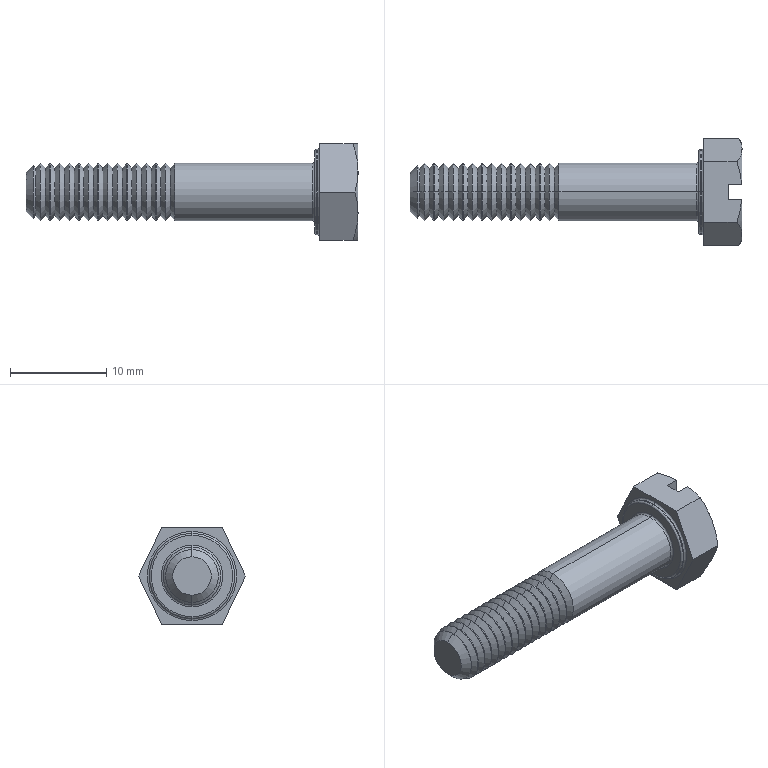Part | SolidWorks | features BaseBody 1 | 1 solid | 124 faces | box 34.5 x 11.106 x 10 mm | volume 1128 mm3 | cone 68 | cylinder 32 | plane 18 | torus 6 | commonest cylinder face diameters 6 x30 8.88 x2